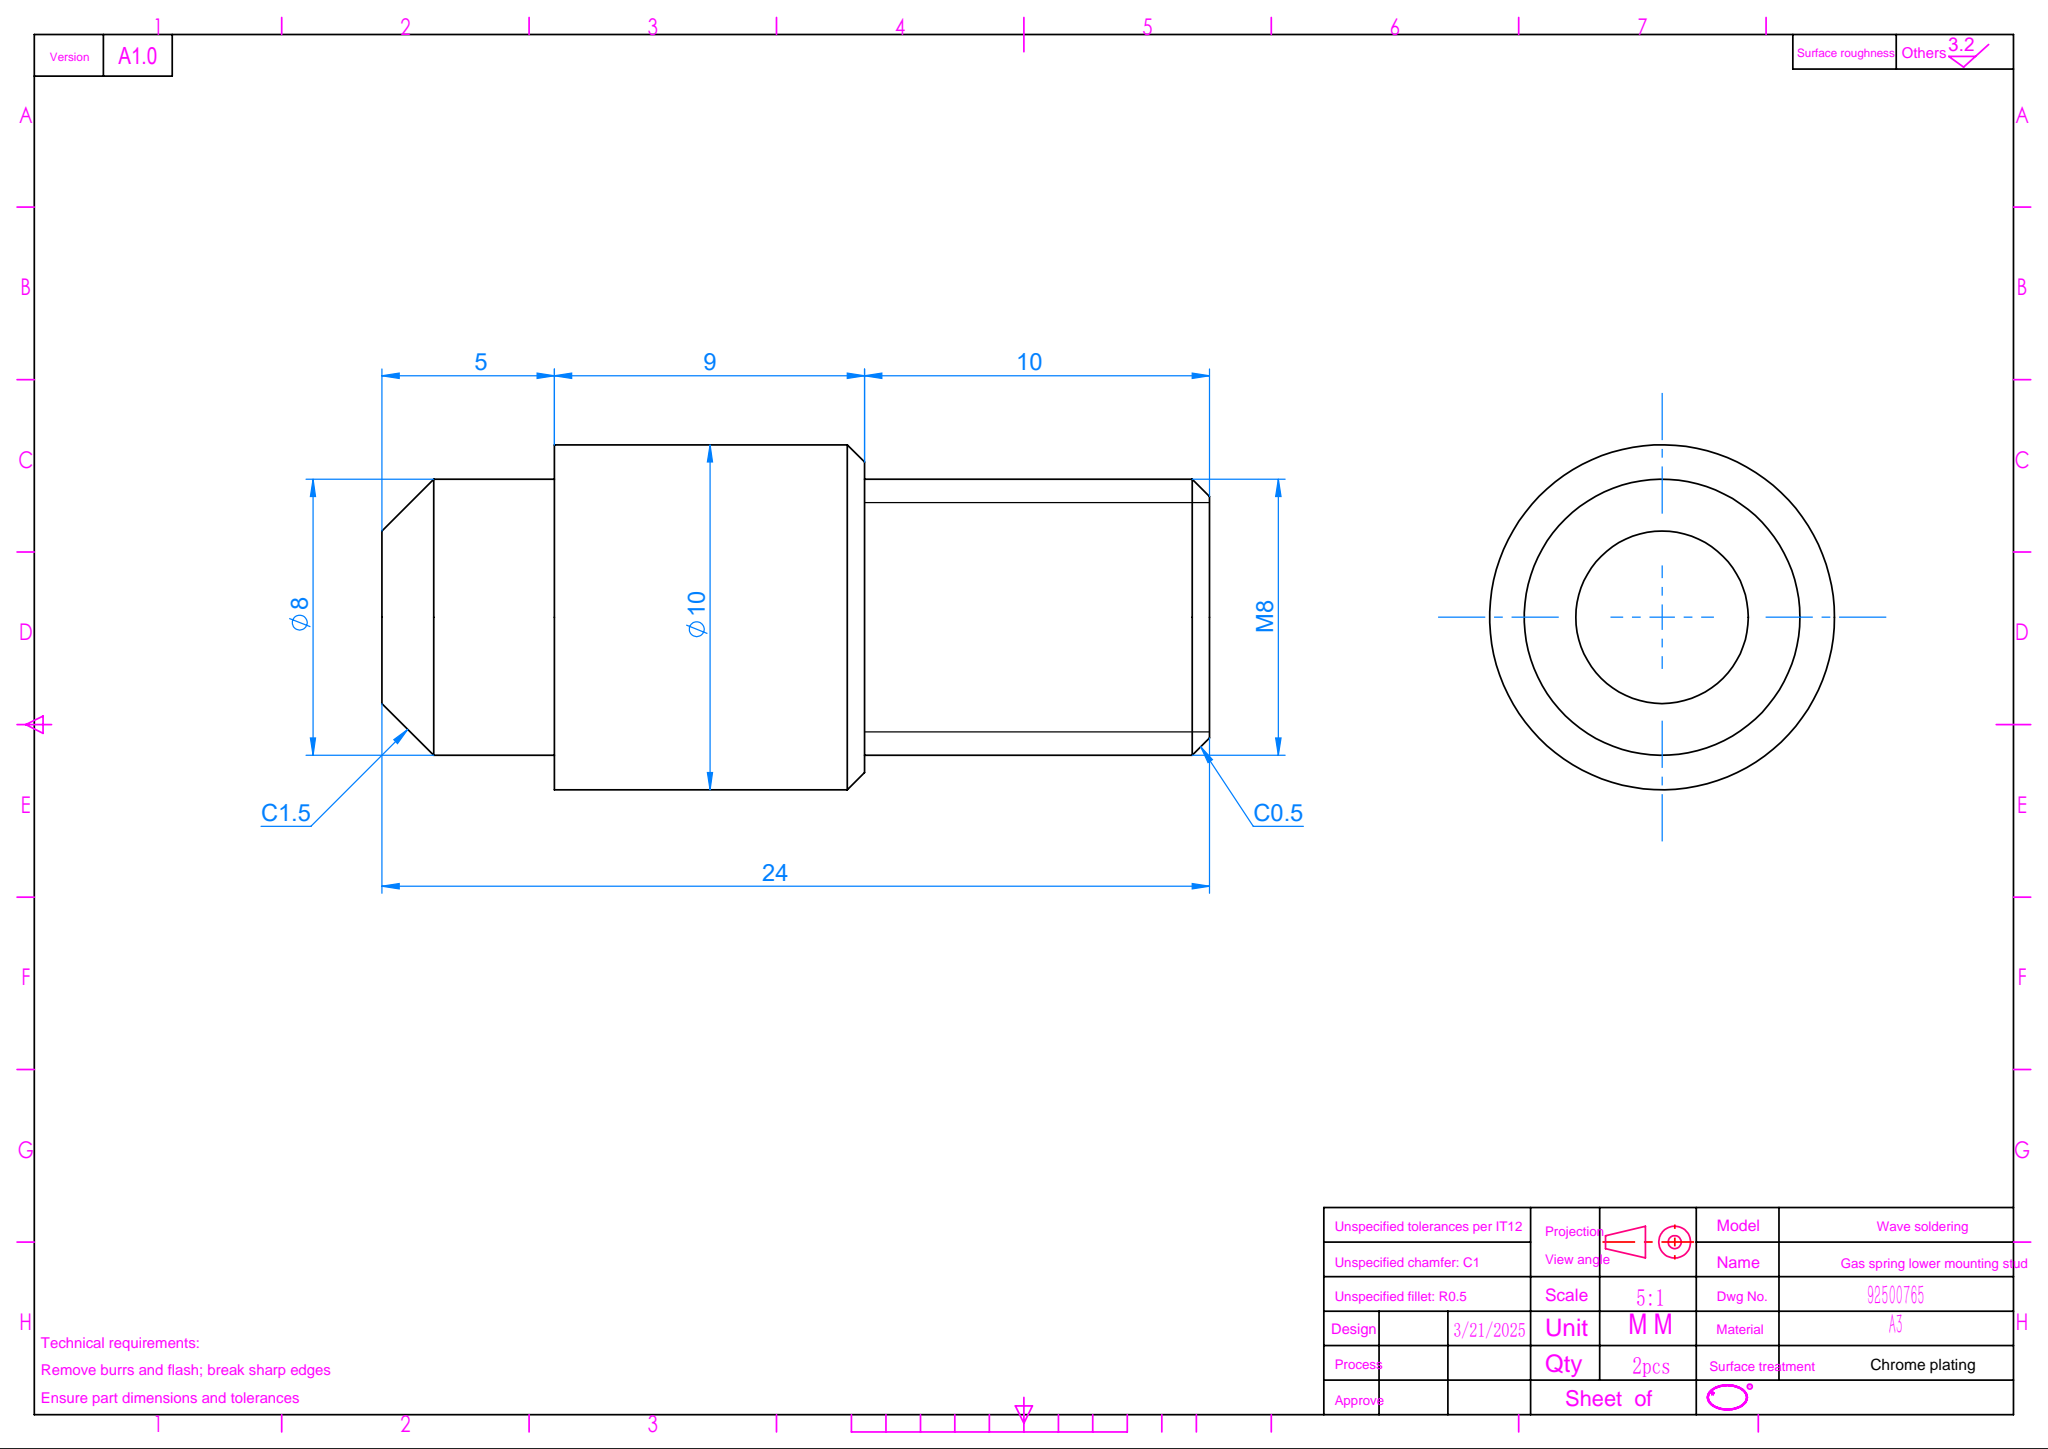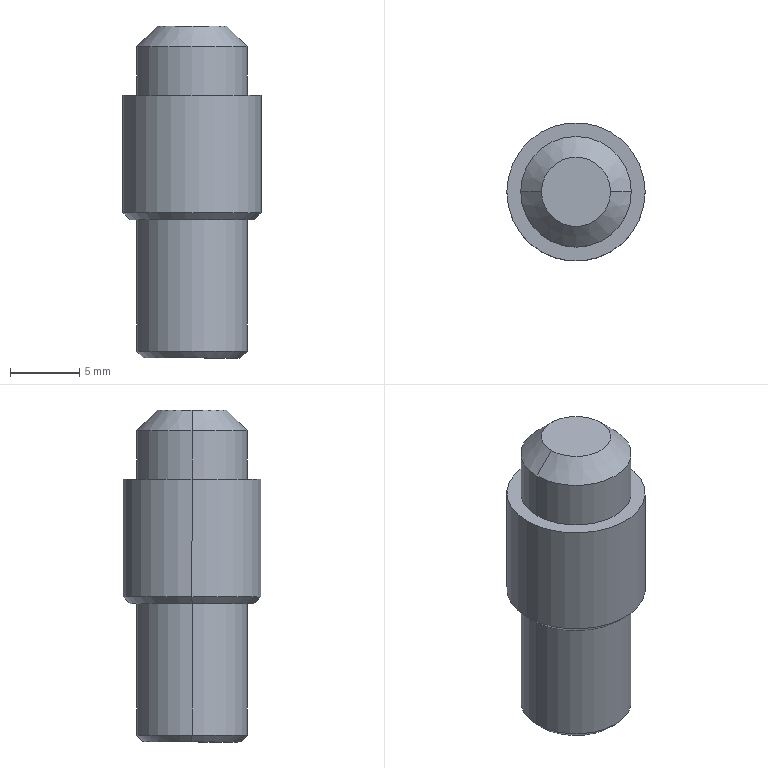Part | SolidWorks | features ICE 3, Chamfer 2, MoveFace 1, RefAxis 1 | 1 solid | 16 faces | box 10 x 10 x 24 mm | volume 1429 mm3 | cone 6 | cylinder 6 | plane 4 | commonest cylinder face diameters 8 x4 10 x2
STEP:
#1=CARTESIAN_POINT('',(-3.5,0.,0.));
#2=VERTEX_POINT('',#1);
#3=CARTESIAN_POINT('',(3.5,0.,0.));
#4=VERTEX_POINT('',#3);
#5=CARTESIAN_POINT('',(0.,0.,0.));
#6=DIRECTION('',(0.,0.,-1.));
#7=DIRECTION('',(1.,0.,0.));
#8=AXIS2_PLACEMENT_3D('',#5,#6,#7);
#9=CIRCLE('',#8,3.5);
#10=EDGE_CURVE('',#2,#4,#9,.T.);
#11=ORIENTED_EDGE('',*,*,#10,.F.);
#12=CARTESIAN_POINT('',(-4.,0.,0.5));
#13=VERTEX_POINT('',#12);
#14=CARTESIAN_POINT('',(-3.5,0.,0.));
#15=DIRECTION('',(-0.7071,0.,0.7071));
#16=VECTOR('',#15,1000.);
#17=LINE('',#14,#16);
#18=EDGE_CURVE('',#2,#13,#17,.T.);
#19=ORIENTED_EDGE('',*,*,#18,.T.);
#20=CARTESIAN_POINT('',(4.,0.,0.5));
#21=VERTEX_POINT('',#20);
#22=CARTESIAN_POINT('',(0.,0.,0.5));
#23=DIRECTION('',(0.,0.,1.));
#24=DIRECTION('',(1.,0.,0.));
#25=AXIS2_PLACEMENT_3D('',#22,#23,#24);
#26=CIRCLE('',#25,4.);
#27=EDGE_CURVE('',#21,#13,#26,.T.);
#28=ORIENTED_EDGE('',*,*,#27,.F.);
#29=CARTESIAN_POINT('',(3.5,0.,0.));
#30=DIRECTION('',(0.7071,0.,0.7071));
#31=VECTOR('',#30,1000.);
#32=LINE('',#29,#31);
#33=EDGE_CURVE('',#4,#21,#32,.T.);
#34=ORIENTED_EDGE('',*,*,#33,.F.);
#35=EDGE_LOOP('',(#11,#19,#28,#34));
#36=FACE_OUTER_BOUND('',#35,.T.);
#37=CARTESIAN_POINT('',(0.,0.,0.));
#38=DIRECTION('',(0.,0.,1.));
#39=DIRECTION('',(1.,0.,0.));
#40=AXIS2_PLACEMENT_3D('',#37,#38,#39);
#41=CONICAL_SURFACE('',#40,3.5,0.7854);
#42=ADVANCED_FACE('',(#36),#41,.T.);
#43=CARTESIAN_POINT('',(-4.5,0.,10.));
#44=VERTEX_POINT('',#43);
#45=CARTESIAN_POINT('',(4.5,0.,10.));
#46=VERTEX_POINT('',#45);
#47=CARTESIAN_POINT('',(0.,0.,10.));
#48=DIRECTION('',(0.,0.,-1.));
#49=DIRECTION('',(-1.,0.,0.));
#50=AXIS2_PLACEMENT_3D('',#47,#48,#49);
#51=CIRCLE('',#50,4.5);
#52=EDGE_CURVE('',#44,#46,#51,.T.);
#53=ORIENTED_EDGE('',*,*,#52,.F.);
#54=CARTESIAN_POINT('',(-5.,0.,10.5));
#55=VERTEX_POINT('',#54);
#56=CARTESIAN_POINT('',(-4.5,0.,10.));
#57=DIRECTION('',(-0.7071,0.,0.7071));
#58=VECTOR('',#57,1000.);
#59=LINE('',#56,#58);
#60=EDGE_CURVE('',#44,#55,#59,.T.);
#61=ORIENTED_EDGE('',*,*,#60,.T.);
#62=CARTESIAN_POINT('',(5.,0.,10.5));
#63=VERTEX_POINT('',#62);
#64=CARTESIAN_POINT('',(0.,0.,10.5));
#65=DIRECTION('',(0.,0.,1.));
#66=DIRECTION('',(-1.,0.,0.));
#67=AXIS2_PLACEMENT_3D('',#64,#65,#66);
#68=CIRCLE('',#67,5.);
#69=EDGE_CURVE('',#63,#55,#68,.T.);
#70=ORIENTED_EDGE('',*,*,#69,.F.);
#71=CARTESIAN_POINT('',(4.5,0.,10.));
#72=DIRECTION('',(0.7071,0.,0.7071));
#73=VECTOR('',#72,1000.);
#74=LINE('',#71,#73);
#75=EDGE_CURVE('',#46,#63,#74,.T.);
#76=ORIENTED_EDGE('',*,*,#75,.F.);
#77=EDGE_LOOP('',(#53,#61,#70,#76));
#78=FACE_OUTER_BOUND('',#77,.T.);
#79=CARTESIAN_POINT('',(0.,0.,10.));
#80=DIRECTION('',(0.,0.,1.));
#81=DIRECTION('',(1.,0.,0.));
#82=AXIS2_PLACEMENT_3D('',#79,#80,#81);
#83=CONICAL_SURFACE('',#82,4.5,0.7854);
#84=ADVANCED_FACE('',(#78),#83,.T.);
#85=CARTESIAN_POINT('',(2.5,0.,24.));
#86=VERTEX_POINT('',#85);
#87=CARTESIAN_POINT('',(-2.5,0.,24.));
#88=VERTEX_POINT('',#87);
#89=CARTESIAN_POINT('',(0.,0.,24.));
#90=DIRECTION('',(0.,0.,1.));
#91=DIRECTION('',(1.,0.,0.));
#92=AXIS2_PLACEMENT_3D('',#89,#90,#91);
#93=CIRCLE('',#92,2.5);
#94=EDGE_CURVE('',#86,#88,#93,.T.);
#95=ORIENTED_EDGE('',*,*,#94,.F.);
#96=CARTESIAN_POINT('',(4.,0.,22.5));
#97=VERTEX_POINT('',#96);
#98=CARTESIAN_POINT('',(2.5,0.,24.));
#99=DIRECTION('',(0.7071,0.,-0.7071));
#100=VECTOR('',#99,1000.);
#101=LINE('',#98,#100);
#102=EDGE_CURVE('',#86,#97,#101,.T.);
#103=ORIENTED_EDGE('',*,*,#102,.T.);
#104=CARTESIAN_POINT('',(-4.,0.,22.5));
#105=VERTEX_POINT('',#104);
#106=CARTESIAN_POINT('',(0.,0.,22.5));
#107=DIRECTION('',(0.,0.,-1.));
#108=DIRECTION('',(1.,0.,0.));
#109=AXIS2_PLACEMENT_3D('',#106,#107,#108);
#110=CIRCLE('',#109,4.);
#111=EDGE_CURVE('',#105,#97,#110,.T.);
#112=ORIENTED_EDGE('',*,*,#111,.F.);
#113=CARTESIAN_POINT('',(-2.5,0.,24.));
#114=DIRECTION('',(-0.7071,0.,-0.7071));
#115=VECTOR('',#114,1000.);
#116=LINE('',#113,#115);
#117=EDGE_CURVE('',#88,#105,#116,.T.);
#118=ORIENTED_EDGE('',*,*,#117,.F.);
#119=EDGE_LOOP('',(#95,#103,#112,#118));
#120=FACE_OUTER_BOUND('',#119,.T.);
#121=CARTESIAN_POINT('',(0.,0.,24.));
#122=DIRECTION('',(0.,0.,-1.));
#123=DIRECTION('',(-1.,0.,0.));
#124=AXIS2_PLACEMENT_3D('',#121,#122,#123);
#125=CONICAL_SURFACE('',#124,2.5,0.7854);
#126=ADVANCED_FACE('',(#120),#125,.T.);
#127=CARTESIAN_POINT('',(-4.,0.,10.));
#128=VERTEX_POINT('',#127);
#129=CARTESIAN_POINT('',(4.,0.,10.));
#130=VERTEX_POINT('',#129);
#131=CARTESIAN_POINT('',(0.,0.,10.));
#132=DIRECTION('',(0.,0.,-1.));
#133=DIRECTION('',(-1.,0.,0.));
#134=AXIS2_PLACEMENT_3D('',#131,#132,#133);
#135=CIRCLE('',#134,4.);
#136=EDGE_CURVE('',#128,#130,#135,.T.);
#137=ORIENTED_EDGE('',*,*,#136,.T.);
#138=CARTESIAN_POINT('',(4.,0.,10.));
#139=DIRECTION('',(0.,0.,-1.));
#140=VECTOR('',#139,1000.);
#141=LINE('',#138,#140);
#142=EDGE_CURVE('',#130,#21,#141,.T.);
#143=ORIENTED_EDGE('',*,*,#142,.T.);
#144=ORIENTED_EDGE('',*,*,#27,.T.);
#145=CARTESIAN_POINT('',(-4.,0.,10.));
#146=DIRECTION('',(0.,0.,-1.));
#147=VECTOR('',#146,1000.);
#148=LINE('',#145,#147);
#149=EDGE_CURVE('',#128,#13,#148,.T.);
#150=ORIENTED_EDGE('',*,*,#149,.F.);
#151=EDGE_LOOP('',(#137,#143,#144,#150));
#152=FACE_OUTER_BOUND('',#151,.T.);
#153=CARTESIAN_POINT('',(0.,0.,10.));
#154=DIRECTION('',(0.,0.,-1.));
#155=DIRECTION('',(-1.,0.,0.));
#156=AXIS2_PLACEMENT_3D('',#153,#154,#155);
#157=CYLINDRICAL_SURFACE('',#156,4.);
#158=ADVANCED_FACE('',(#152),#157,.T.);
#159=CARTESIAN_POINT('',(4.,0.,19.));
#160=VERTEX_POINT('',#159);
#161=CARTESIAN_POINT('',(-4.,0.,19.));
#162=VERTEX_POINT('',#161);
#163=CARTESIAN_POINT('',(0.,0.,19.));
#164=DIRECTION('',(0.,0.,1.));
#165=DIRECTION('',(1.,0.,0.));
#166=AXIS2_PLACEMENT_3D('',#163,#164,#165);
#167=CIRCLE('',#166,4.);
#168=EDGE_CURVE('',#160,#162,#167,.T.);
#169=ORIENTED_EDGE('',*,*,#168,.T.);
#170=CARTESIAN_POINT('',(-4.,0.,19.));
#171=DIRECTION('',(0.,0.,1.));
#172=VECTOR('',#171,1000.);
#173=LINE('',#170,#172);
#174=EDGE_CURVE('',#162,#105,#173,.T.);
#175=ORIENTED_EDGE('',*,*,#174,.T.);
#176=ORIENTED_EDGE('',*,*,#111,.T.);
#177=CARTESIAN_POINT('',(4.,0.,19.));
#178=DIRECTION('',(0.,0.,1.));
#179=VECTOR('',#178,1000.);
#180=LINE('',#177,#179);
#181=EDGE_CURVE('',#160,#97,#180,.T.);
#182=ORIENTED_EDGE('',*,*,#181,.F.);
#183=EDGE_LOOP('',(#169,#175,#176,#182));
#184=FACE_OUTER_BOUND('',#183,.T.);
#185=CARTESIAN_POINT('',(0.,0.,19.));
#186=DIRECTION('',(0.,0.,1.));
#187=DIRECTION('',(1.,0.,0.));
#188=AXIS2_PLACEMENT_3D('',#185,#186,#187);
#189=CYLINDRICAL_SURFACE('',#188,4.);
#190=ADVANCED_FACE('',(#184),#189,.T.);
#191=CARTESIAN_POINT('',(5.,0.,19.));
#192=VERTEX_POINT('',#191);
#193=CARTESIAN_POINT('',(-5.,0.,19.));
#194=VERTEX_POINT('',#193);
#195=CARTESIAN_POINT('',(0.,0.,19.));
#196=DIRECTION('',(0.,0.,1.));
#197=DIRECTION('',(1.,0.,0.));
#198=AXIS2_PLACEMENT_3D('',#195,#196,#197);
#199=CIRCLE('',#198,5.);
#200=EDGE_CURVE('',#192,#194,#199,.T.);
#201=ORIENTED_EDGE('',*,*,#200,.F.);
#202=CARTESIAN_POINT('',(5.,0.,22.));
#203=DIRECTION('',(0.,0.,-1.));
#204=VECTOR('',#203,1000.);
#205=LINE('',#202,#204);
#206=EDGE_CURVE('',#192,#63,#205,.T.);
#207=ORIENTED_EDGE('',*,*,#206,.T.);
#208=ORIENTED_EDGE('',*,*,#69,.T.);
#209=CARTESIAN_POINT('',(-5.,0.,22.));
#210=DIRECTION('',(0.,0.,-1.));
#211=VECTOR('',#210,1000.);
#212=LINE('',#209,#211);
#213=EDGE_CURVE('',#194,#55,#212,.T.);
#214=ORIENTED_EDGE('',*,*,#213,.F.);
#215=EDGE_LOOP('',(#201,#207,#208,#214));
#216=FACE_OUTER_BOUND('',#215,.T.);
#217=CARTESIAN_POINT('',(0.,0.,22.));
#218=DIRECTION('',(0.,0.,-1.));
#219=DIRECTION('',(-1.,0.,0.));
#220=AXIS2_PLACEMENT_3D('',#217,#218,#219);
#221=CYLINDRICAL_SURFACE('',#220,5.);
#222=ADVANCED_FACE('',(#216),#221,.T.);
#223=ORIENTED_EDGE('',*,*,#206,.F.);
#224=CARTESIAN_POINT('',(0.,0.,19.));
#225=DIRECTION('',(0.,0.,1.));
#226=DIRECTION('',(1.,0.,0.));
#227=AXIS2_PLACEMENT_3D('',#224,#225,#226);
#228=CIRCLE('',#227,5.);
#229=EDGE_CURVE('',#194,#192,#228,.T.);
#230=ORIENTED_EDGE('',*,*,#229,.F.);
#231=ORIENTED_EDGE('',*,*,#213,.T.);
#232=CARTESIAN_POINT('',(0.,0.,10.5));
#233=DIRECTION('',(0.,0.,1.));
#234=DIRECTION('',(-1.,0.,0.));
#235=AXIS2_PLACEMENT_3D('',#232,#233,#234);
#236=CIRCLE('',#235,5.);
#237=EDGE_CURVE('',#55,#63,#236,.T.);
#238=ORIENTED_EDGE('',*,*,#237,.T.);
#239=EDGE_LOOP('',(#223,#230,#231,#238));
#240=FACE_OUTER_BOUND('',#239,.T.);
#241=CARTESIAN_POINT('',(0.,0.,22.));
#242=DIRECTION('',(0.,0.,-1.));
#243=DIRECTION('',(-1.,0.,0.));
#244=AXIS2_PLACEMENT_3D('',#241,#242,#243);
#245=CYLINDRICAL_SURFACE('',#244,5.);
#246=ADVANCED_FACE('',(#240),#245,.T.);
#247=ORIENTED_EDGE('',*,*,#168,.F.);
#248=CARTESIAN_POINT('',(0.,0.,19.));
#249=DIRECTION('',(0.,0.,1.));
#250=DIRECTION('',(1.,0.,0.));
#251=AXIS2_PLACEMENT_3D('',#248,#249,#250);
#252=CIRCLE('',#251,4.);
#253=EDGE_CURVE('',#162,#160,#252,.T.);
#254=ORIENTED_EDGE('',*,*,#253,.F.);
#255=EDGE_LOOP('',(#247,#254));
#256=FACE_BOUND('',#255,.T.);
#257=ORIENTED_EDGE('',*,*,#229,.T.);
#258=ORIENTED_EDGE('',*,*,#200,.T.);
#259=EDGE_LOOP('',(#257,#258));
#260=FACE_OUTER_BOUND('',#259,.T.);
#261=CARTESIAN_POINT('',(0.,0.,19.));
#262=DIRECTION('',(0.,0.,1.));
#263=DIRECTION('',(1.,0.,0.));
#264=AXIS2_PLACEMENT_3D('',#261,#262,#263);
#265=PLANE('',#264);
#266=ADVANCED_FACE('',(#256,#260),#265,.T.);
#267=ORIENTED_EDGE('',*,*,#174,.F.);
#268=ORIENTED_EDGE('',*,*,#253,.T.);
#269=ORIENTED_EDGE('',*,*,#181,.T.);
#270=CARTESIAN_POINT('',(0.,0.,22.5));
#271=DIRECTION('',(0.,0.,-1.));
#272=DIRECTION('',(1.,0.,0.));
#273=AXIS2_PLACEMENT_3D('',#270,#271,#272);
#274=CIRCLE('',#273,4.);
#275=EDGE_CURVE('',#97,#105,#274,.T.);
#276=ORIENTED_EDGE('',*,*,#275,.T.);
#277=EDGE_LOOP('',(#267,#268,#269,#276));
#278=FACE_OUTER_BOUND('',#277,.T.);
#279=CARTESIAN_POINT('',(0.,0.,19.));
#280=DIRECTION('',(0.,0.,1.));
#281=DIRECTION('',(1.,0.,0.));
#282=AXIS2_PLACEMENT_3D('',#279,#280,#281);
#283=CYLINDRICAL_SURFACE('',#282,4.);
#284=ADVANCED_FACE('',(#278),#283,.T.);
#285=CARTESIAN_POINT('',(0.,0.,24.));
#286=DIRECTION('',(0.,0.,1.));
#287=DIRECTION('',(1.,0.,0.));
#288=AXIS2_PLACEMENT_3D('',#285,#286,#287);
#289=CIRCLE('',#288,2.5);
#290=EDGE_CURVE('',#88,#86,#289,.T.);
#291=ORIENTED_EDGE('',*,*,#290,.T.);
#292=ORIENTED_EDGE('',*,*,#94,.T.);
#293=EDGE_LOOP('',(#291,#292));
#294=FACE_OUTER_BOUND('',#293,.T.);
#295=CARTESIAN_POINT('',(0.,0.,24.));
#296=DIRECTION('',(0.,0.,1.));
#297=DIRECTION('',(1.,0.,0.));
#298=AXIS2_PLACEMENT_3D('',#295,#296,#297);
#299=PLANE('',#298);
#300=ADVANCED_FACE('',(#294),#299,.T.);
#301=CARTESIAN_POINT('',(0.,0.,10.));
#302=DIRECTION('',(0.,0.,-1.));
#303=DIRECTION('',(-1.,0.,0.));
#304=AXIS2_PLACEMENT_3D('',#301,#302,#303);
#305=CIRCLE('',#304,4.5);
#306=EDGE_CURVE('',#46,#44,#305,.T.);
#307=ORIENTED_EDGE('',*,*,#306,.T.);
#308=ORIENTED_EDGE('',*,*,#52,.T.);
#309=EDGE_LOOP('',(#307,#308));
#310=FACE_OUTER_BOUND('',#309,.T.);
#311=ORIENTED_EDGE('',*,*,#136,.F.);
#312=CARTESIAN_POINT('',(0.,0.,10.));
#313=DIRECTION('',(0.,0.,-1.));
#314=DIRECTION('',(-1.,0.,0.));
#315=AXIS2_PLACEMENT_3D('',#312,#313,#314);
#316=CIRCLE('',#315,4.);
#317=EDGE_CURVE('',#130,#128,#316,.T.);
#318=ORIENTED_EDGE('',*,*,#317,.F.);
#319=EDGE_LOOP('',(#311,#318));
#320=FACE_BOUND('',#319,.T.);
#321=CARTESIAN_POINT('',(0.,0.,10.));
#322=DIRECTION('',(0.,0.,-1.));
#323=DIRECTION('',(-1.,0.,0.));
#324=AXIS2_PLACEMENT_3D('',#321,#322,#323);
#325=PLANE('',#324);
#326=ADVANCED_FACE('',(#310,#320),#325,.T.);
#327=ORIENTED_EDGE('',*,*,#142,.F.);
#328=ORIENTED_EDGE('',*,*,#317,.T.);
#329=ORIENTED_EDGE('',*,*,#149,.T.);
#330=CARTESIAN_POINT('',(0.,0.,0.5));
#331=DIRECTION('',(0.,0.,1.));
#332=DIRECTION('',(1.,0.,0.));
#333=AXIS2_PLACEMENT_3D('',#330,#331,#332);
#334=CIRCLE('',#333,4.);
#335=EDGE_CURVE('',#13,#21,#334,.T.);
#336=ORIENTED_EDGE('',*,*,#335,.T.);
#337=EDGE_LOOP('',(#327,#328,#329,#336));
#338=FACE_OUTER_BOUND('',#337,.T.);
#339=CARTESIAN_POINT('',(0.,0.,10.));
#340=DIRECTION('',(0.,0.,-1.));
#341=DIRECTION('',(-1.,0.,0.));
#342=AXIS2_PLACEMENT_3D('',#339,#340,#341);
#343=CYLINDRICAL_SURFACE('',#342,4.);
#344=ADVANCED_FACE('',(#338),#343,.T.);
#345=CARTESIAN_POINT('',(0.,0.,0.));
#346=DIRECTION('',(0.,0.,-1.));
#347=DIRECTION('',(1.,0.,0.));
#348=AXIS2_PLACEMENT_3D('',#345,#346,#347);
#349=CIRCLE('',#348,3.5);
#350=EDGE_CURVE('',#4,#2,#349,.T.);
#351=ORIENTED_EDGE('',*,*,#350,.T.);
#352=ORIENTED_EDGE('',*,*,#10,.T.);
#353=EDGE_LOOP('',(#351,#352));
#354=FACE_OUTER_BOUND('',#353,.T.);
#355=CARTESIAN_POINT('',(0.,0.,0.));
#356=DIRECTION('',(0.,0.,1.));
#357=DIRECTION('',(1.,0.,0.));
#358=AXIS2_PLACEMENT_3D('',#355,#356,#357);
#359=PLANE('',#358);
#360=ADVANCED_FACE('',(#354),#359,.F.);
#361=ORIENTED_EDGE('',*,*,#102,.F.);
#362=ORIENTED_EDGE('',*,*,#290,.F.);
#363=ORIENTED_EDGE('',*,*,#117,.T.);
#364=ORIENTED_EDGE('',*,*,#275,.F.);
#365=EDGE_LOOP('',(#361,#362,#363,#364));
#366=FACE_OUTER_BOUND('',#365,.T.);
#367=CARTESIAN_POINT('',(0.,0.,24.));
#368=DIRECTION('',(0.,0.,-1.));
#369=DIRECTION('',(-1.,0.,0.));
#370=AXIS2_PLACEMENT_3D('',#367,#368,#369);
#371=CONICAL_SURFACE('',#370,2.5,0.7854);
#372=ADVANCED_FACE('',(#366),#371,.T.);
#373=ORIENTED_EDGE('',*,*,#60,.F.);
#374=ORIENTED_EDGE('',*,*,#306,.F.);
#375=ORIENTED_EDGE('',*,*,#75,.T.);
#376=ORIENTED_EDGE('',*,*,#237,.F.);
#377=EDGE_LOOP('',(#373,#374,#375,#376));
#378=FACE_OUTER_BOUND('',#377,.T.);
#379=CARTESIAN_POINT('',(0.,0.,10.));
#380=DIRECTION('',(0.,0.,1.));
#381=DIRECTION('',(1.,0.,0.));
#382=AXIS2_PLACEMENT_3D('',#379,#380,#381);
#383=CONICAL_SURFACE('',#382,4.5,0.7854);
#384=ADVANCED_FACE('',(#378),#383,.T.);
#385=ORIENTED_EDGE('',*,*,#18,.F.);
#386=ORIENTED_EDGE('',*,*,#350,.F.);
#387=ORIENTED_EDGE('',*,*,#33,.T.);
#388=ORIENTED_EDGE('',*,*,#335,.F.);
#389=EDGE_LOOP('',(#385,#386,#387,#388));
#390=FACE_OUTER_BOUND('',#389,.T.);
#391=CARTESIAN_POINT('',(0.,0.,0.));
#392=DIRECTION('',(0.,0.,1.));
#393=DIRECTION('',(1.,0.,0.));
#394=AXIS2_PLACEMENT_3D('',#391,#392,#393);
#395=CONICAL_SURFACE('',#394,3.5,0.7854);
#396=ADVANCED_FACE('',(#390),#395,.T.);
#397=CLOSED_SHELL('',(#42,#84,#126,#158,#190,#222,#246,#266,#284,#300,#326,#344,#360,#372,#384,#396));
#398=MANIFOLD_SOLID_BREP('',#397);
#399=CARTESIAN_POINT('',(0.,0.,0.));
#400=DIRECTION('',(0.,0.,1.));
#401=DIRECTION('',(1.,0.,0.));
#402=AXIS2_PLACEMENT_3D('',#399,#400,#401);
#403=(LENGTH_UNIT()NAMED_UNIT(*)SI_UNIT(.MILLI.,.METRE.));
#404=UNCERTAINTY_MEASURE_WITH_UNIT(LENGTH_MEASURE(0.00001),#403,'','');
#405=(NAMED_UNIT(*)PLANE_ANGLE_UNIT()SI_UNIT($,.RADIAN.));
#406=(NAMED_UNIT(*)SI_UNIT($,.STERADIAN.)SOLID_ANGLE_UNIT());
#407=(GEOMETRIC_REPRESENTATION_CONTEXT(3)GLOBAL_UNCERTAINTY_ASSIGNED_CONTEXT((#404))GLOBAL_UNIT_ASSIGNED_CONTEXT((#403,#405,#406))REPRESENTATION_CONTEXT('',''));
#408=ADVANCED_BREP_SHAPE_REPRESENTATION('',(#398,#402),#407);